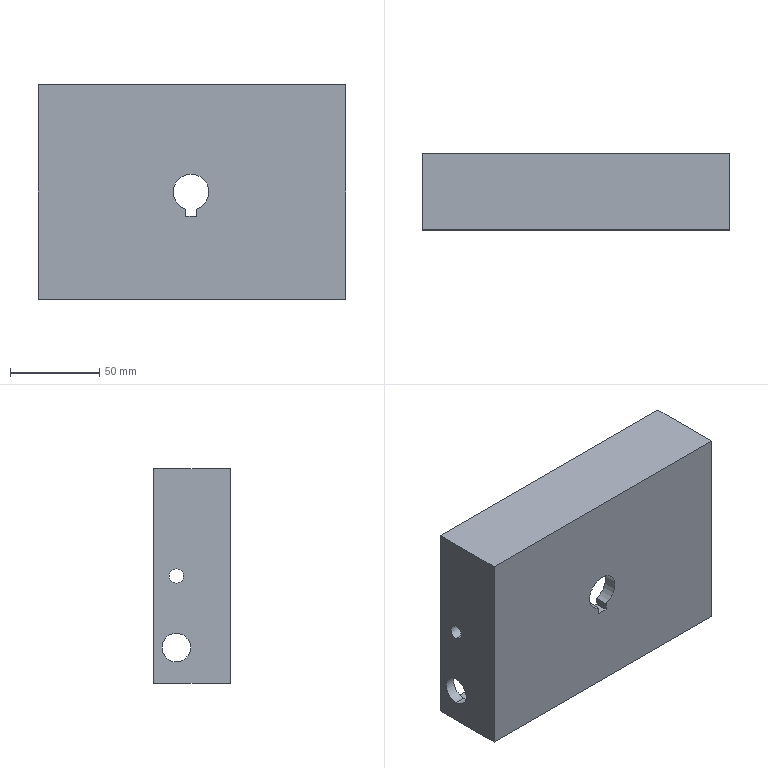Part | SolidWorks | features ICE 3, Extrusion 1 | 1 solid | 23 faces | box 172 x 42.5 x 120 mm | volume 233262 mm3 | plane 14 | cylinder 9 | commonest cylinder face diameters 8 x4 16 x4 20 x1
STEP:
#1=CARTESIAN_POINT('',(86.,8.75,56.));
#2=VERTEX_POINT('',#1);
#3=CARTESIAN_POINT('',(86.,8.75,64.));
#4=VERTEX_POINT('',#3);
#5=CARTESIAN_POINT('',(86.,8.75,60.));
#6=DIRECTION('',(-1.,0.,0.));
#7=DIRECTION('',(0.,0.,1.));
#8=AXIS2_PLACEMENT_3D('',#5,#6,#7);
#9=CIRCLE('',#8,4.);
#10=EDGE_CURVE('',#2,#4,#9,.T.);
#11=ORIENTED_EDGE('',*,*,#10,.F.);
#12=CARTESIAN_POINT('',(80.,8.75,56.));
#13=VERTEX_POINT('',#12);
#14=CARTESIAN_POINT('',(86.,8.75,56.));
#15=DIRECTION('',(-1.,0.,0.));
#16=VECTOR('',#15,1000.);
#17=LINE('',#14,#16);
#18=EDGE_CURVE('',#2,#13,#17,.T.);
#19=ORIENTED_EDGE('',*,*,#18,.T.);
#20=CARTESIAN_POINT('',(80.,8.75,64.));
#21=VERTEX_POINT('',#20);
#22=CARTESIAN_POINT('',(80.,8.75,60.));
#23=DIRECTION('',(1.,0.,0.));
#24=DIRECTION('',(0.,0.,-1.));
#25=AXIS2_PLACEMENT_3D('',#22,#23,#24);
#26=CIRCLE('',#25,4.);
#27=EDGE_CURVE('',#21,#13,#26,.T.);
#28=ORIENTED_EDGE('',*,*,#27,.F.);
#29=CARTESIAN_POINT('',(86.,8.75,64.));
#30=DIRECTION('',(-1.,0.,0.));
#31=VECTOR('',#30,1000.);
#32=LINE('',#29,#31);
#33=EDGE_CURVE('',#4,#21,#32,.T.);
#34=ORIENTED_EDGE('',*,*,#33,.F.);
#35=EDGE_LOOP('',(#11,#19,#28,#34));
#36=FACE_OUTER_BOUND('',#35,.T.);
#37=CARTESIAN_POINT('',(86.,8.75,60.));
#38=DIRECTION('',(-1.,0.,0.));
#39=DIRECTION('',(0.,0.,1.));
#40=AXIS2_PLACEMENT_3D('',#37,#38,#39);
#41=CYLINDRICAL_SURFACE('',#40,4.);
#42=ADVANCED_FACE('',(#36),#41,.F.);
#43=CARTESIAN_POINT('',(86.,8.75,12.));
#44=VERTEX_POINT('',#43);
#45=CARTESIAN_POINT('',(86.,8.75,28.));
#46=VERTEX_POINT('',#45);
#47=CARTESIAN_POINT('',(86.,8.75,20.));
#48=DIRECTION('',(-1.,0.,0.));
#49=DIRECTION('',(0.,0.,1.));
#50=AXIS2_PLACEMENT_3D('',#47,#48,#49);
#51=CIRCLE('',#50,8.);
#52=EDGE_CURVE('',#44,#46,#51,.T.);
#53=ORIENTED_EDGE('',*,*,#52,.F.);
#54=CARTESIAN_POINT('',(80.,8.75,12.));
#55=VERTEX_POINT('',#54);
#56=CARTESIAN_POINT('',(86.,8.75,12.));
#57=DIRECTION('',(-1.,0.,0.));
#58=VECTOR('',#57,1000.);
#59=LINE('',#56,#58);
#60=EDGE_CURVE('',#44,#55,#59,.T.);
#61=ORIENTED_EDGE('',*,*,#60,.T.);
#62=CARTESIAN_POINT('',(80.,8.75,28.));
#63=VERTEX_POINT('',#62);
#64=CARTESIAN_POINT('',(80.,8.75,20.));
#65=DIRECTION('',(1.,0.,0.));
#66=DIRECTION('',(0.,0.,-1.));
#67=AXIS2_PLACEMENT_3D('',#64,#65,#66);
#68=CIRCLE('',#67,8.);
#69=EDGE_CURVE('',#63,#55,#68,.T.);
#70=ORIENTED_EDGE('',*,*,#69,.F.);
#71=CARTESIAN_POINT('',(86.,8.75,28.));
#72=DIRECTION('',(-1.,0.,0.));
#73=VECTOR('',#72,1000.);
#74=LINE('',#71,#73);
#75=EDGE_CURVE('',#46,#63,#74,.T.);
#76=ORIENTED_EDGE('',*,*,#75,.F.);
#77=EDGE_LOOP('',(#53,#61,#70,#76));
#78=FACE_OUTER_BOUND('',#77,.T.);
#79=CARTESIAN_POINT('',(86.,8.75,20.));
#80=DIRECTION('',(-1.,0.,0.));
#81=DIRECTION('',(0.,0.,1.));
#82=AXIS2_PLACEMENT_3D('',#79,#80,#81);
#83=CYLINDRICAL_SURFACE('',#82,8.);
#84=ADVANCED_FACE('',(#78),#83,.F.);
#85=CARTESIAN_POINT('',(-80.,8.75,56.));
#86=VERTEX_POINT('',#85);
#87=CARTESIAN_POINT('',(-80.,8.75,64.));
#88=VERTEX_POINT('',#87);
#89=CARTESIAN_POINT('',(-80.,8.75,60.));
#90=DIRECTION('',(-1.,0.,0.));
#91=DIRECTION('',(0.,0.,1.));
#92=AXIS2_PLACEMENT_3D('',#89,#90,#91);
#93=CIRCLE('',#92,4.);
#94=EDGE_CURVE('',#86,#88,#93,.T.);
#95=ORIENTED_EDGE('',*,*,#94,.F.);
#96=CARTESIAN_POINT('',(-86.,8.75,56.));
#97=VERTEX_POINT('',#96);
#98=CARTESIAN_POINT('',(86.,8.75,56.));
#99=DIRECTION('',(-1.,0.,0.));
#100=VECTOR('',#99,1000.);
#101=LINE('',#98,#100);
#102=EDGE_CURVE('',#86,#97,#101,.T.);
#103=ORIENTED_EDGE('',*,*,#102,.T.);
#104=CARTESIAN_POINT('',(-86.,8.75,64.));
#105=VERTEX_POINT('',#104);
#106=CARTESIAN_POINT('',(-86.,8.75,60.));
#107=DIRECTION('',(-1.,0.,0.));
#108=DIRECTION('',(0.,0.,1.));
#109=AXIS2_PLACEMENT_3D('',#106,#107,#108);
#110=CIRCLE('',#109,4.);
#111=EDGE_CURVE('',#97,#105,#110,.T.);
#112=ORIENTED_EDGE('',*,*,#111,.T.);
#113=CARTESIAN_POINT('',(86.,8.75,64.));
#114=DIRECTION('',(-1.,0.,0.));
#115=VECTOR('',#114,1000.);
#116=LINE('',#113,#115);
#117=EDGE_CURVE('',#88,#105,#116,.T.);
#118=ORIENTED_EDGE('',*,*,#117,.F.);
#119=EDGE_LOOP('',(#95,#103,#112,#118));
#120=FACE_OUTER_BOUND('',#119,.T.);
#121=CARTESIAN_POINT('',(86.,8.75,60.));
#122=DIRECTION('',(-1.,0.,0.));
#123=DIRECTION('',(0.,0.,1.));
#124=AXIS2_PLACEMENT_3D('',#121,#122,#123);
#125=CYLINDRICAL_SURFACE('',#124,4.);
#126=ADVANCED_FACE('',(#120),#125,.F.);
#127=CARTESIAN_POINT('',(-80.,8.75,12.));
#128=VERTEX_POINT('',#127);
#129=CARTESIAN_POINT('',(-80.,8.75,28.));
#130=VERTEX_POINT('',#129);
#131=CARTESIAN_POINT('',(-80.,8.75,20.));
#132=DIRECTION('',(-1.,0.,0.));
#133=DIRECTION('',(0.,0.,1.));
#134=AXIS2_PLACEMENT_3D('',#131,#132,#133);
#135=CIRCLE('',#134,8.);
#136=EDGE_CURVE('',#128,#130,#135,.T.);
#137=ORIENTED_EDGE('',*,*,#136,.F.);
#138=CARTESIAN_POINT('',(-86.,8.75,12.));
#139=VERTEX_POINT('',#138);
#140=CARTESIAN_POINT('',(86.,8.75,12.));
#141=DIRECTION('',(-1.,0.,0.));
#142=VECTOR('',#141,1000.);
#143=LINE('',#140,#142);
#144=EDGE_CURVE('',#128,#139,#143,.T.);
#145=ORIENTED_EDGE('',*,*,#144,.T.);
#146=CARTESIAN_POINT('',(-86.,8.75,28.));
#147=VERTEX_POINT('',#146);
#148=CARTESIAN_POINT('',(-86.,8.75,20.));
#149=DIRECTION('',(-1.,0.,0.));
#150=DIRECTION('',(0.,0.,1.));
#151=AXIS2_PLACEMENT_3D('',#148,#149,#150);
#152=CIRCLE('',#151,8.);
#153=EDGE_CURVE('',#139,#147,#152,.T.);
#154=ORIENTED_EDGE('',*,*,#153,.T.);
#155=CARTESIAN_POINT('',(86.,8.75,28.));
#156=DIRECTION('',(-1.,0.,0.));
#157=VECTOR('',#156,1000.);
#158=LINE('',#155,#157);
#159=EDGE_CURVE('',#130,#147,#158,.T.);
#160=ORIENTED_EDGE('',*,*,#159,.F.);
#161=EDGE_LOOP('',(#137,#145,#154,#160));
#162=FACE_OUTER_BOUND('',#161,.T.);
#163=CARTESIAN_POINT('',(86.,8.75,20.));
#164=DIRECTION('',(-1.,0.,0.));
#165=DIRECTION('',(0.,0.,1.));
#166=AXIS2_PLACEMENT_3D('',#163,#164,#165);
#167=CYLINDRICAL_SURFACE('',#166,8.);
#168=ADVANCED_FACE('',(#162),#167,.F.);
#169=CARTESIAN_POINT('',(86.,8.75,60.));
#170=DIRECTION('',(-1.,0.,0.));
#171=DIRECTION('',(0.,0.,1.));
#172=AXIS2_PLACEMENT_3D('',#169,#170,#171);
#173=CIRCLE('',#172,4.);
#174=EDGE_CURVE('',#4,#2,#173,.T.);
#175=ORIENTED_EDGE('',*,*,#174,.T.);
#176=ORIENTED_EDGE('',*,*,#10,.T.);
#177=EDGE_LOOP('',(#175,#176));
#178=FACE_BOUND('',#177,.T.);
#179=CARTESIAN_POINT('',(86.,8.75,20.));
#180=DIRECTION('',(-1.,0.,0.));
#181=DIRECTION('',(0.,0.,1.));
#182=AXIS2_PLACEMENT_3D('',#179,#180,#181);
#183=CIRCLE('',#182,8.);
#184=EDGE_CURVE('',#46,#44,#183,.T.);
#185=ORIENTED_EDGE('',*,*,#184,.T.);
#186=ORIENTED_EDGE('',*,*,#52,.T.);
#187=EDGE_LOOP('',(#185,#186));
#188=FACE_BOUND('',#187,.T.);
#189=CARTESIAN_POINT('',(86.,-21.25,0.));
#190=VERTEX_POINT('',#189);
#191=CARTESIAN_POINT('',(86.,21.25,0.));
#192=VERTEX_POINT('',#191);
#193=CARTESIAN_POINT('',(86.,-21.25,0.));
#194=DIRECTION('',(0.,1.,0.));
#195=VECTOR('',#194,1000.);
#196=LINE('',#193,#195);
#197=EDGE_CURVE('',#190,#192,#196,.T.);
#198=ORIENTED_EDGE('',*,*,#197,.T.);
#199=CARTESIAN_POINT('',(86.,21.25,120.));
#200=VERTEX_POINT('',#199);
#201=CARTESIAN_POINT('',(86.,21.25,120.));
#202=DIRECTION('',(0.,0.,-1.));
#203=VECTOR('',#202,1000.);
#204=LINE('',#201,#203);
#205=EDGE_CURVE('',#200,#192,#204,.T.);
#206=ORIENTED_EDGE('',*,*,#205,.F.);
#207=CARTESIAN_POINT('',(86.,-21.25,120.));
#208=VERTEX_POINT('',#207);
#209=CARTESIAN_POINT('',(86.,-21.25,120.));
#210=DIRECTION('',(0.,1.,0.));
#211=VECTOR('',#210,1000.);
#212=LINE('',#209,#211);
#213=EDGE_CURVE('',#208,#200,#212,.T.);
#214=ORIENTED_EDGE('',*,*,#213,.F.);
#215=CARTESIAN_POINT('',(86.,-21.25,120.));
#216=DIRECTION('',(0.,0.,-1.));
#217=VECTOR('',#216,1000.);
#218=LINE('',#215,#217);
#219=EDGE_CURVE('',#208,#190,#218,.T.);
#220=ORIENTED_EDGE('',*,*,#219,.T.);
#221=EDGE_LOOP('',(#198,#206,#214,#220));
#222=FACE_OUTER_BOUND('',#221,.T.);
#223=CARTESIAN_POINT('',(86.,-21.25,120.));
#224=DIRECTION('',(-1.,0.,0.));
#225=DIRECTION('',(0.,0.,1.));
#226=AXIS2_PLACEMENT_3D('',#223,#224,#225);
#227=PLANE('',#226);
#228=ADVANCED_FACE('',(#178,#188,#222),#227,.F.);
#229=CARTESIAN_POINT('',(-80.,21.25,3.));
#230=VERTEX_POINT('',#229);
#231=CARTESIAN_POINT('',(-80.,21.25,117.));
#232=VERTEX_POINT('',#231);
#233=CARTESIAN_POINT('',(-80.,21.25,5.));
#234=DIRECTION('',(0.,0.,1.));
#235=VECTOR('',#234,1000.);
#236=LINE('',#233,#235);
#237=EDGE_CURVE('',#230,#232,#236,.T.);
#238=ORIENTED_EDGE('',*,*,#237,.F.);
#239=CARTESIAN_POINT('',(80.,21.25,3.));
#240=VERTEX_POINT('',#239);
#241=CARTESIAN_POINT('',(-80.,21.25,3.));
#242=DIRECTION('',(-1.,0.,0.));
#243=VECTOR('',#242,1000.);
#244=LINE('',#241,#243);
#245=EDGE_CURVE('',#240,#230,#244,.T.);
#246=ORIENTED_EDGE('',*,*,#245,.F.);
#247=CARTESIAN_POINT('',(80.,21.25,117.));
#248=VERTEX_POINT('',#247);
#249=CARTESIAN_POINT('',(80.,21.25,3.));
#250=DIRECTION('',(0.,0.,-1.));
#251=VECTOR('',#250,1000.);
#252=LINE('',#249,#251);
#253=EDGE_CURVE('',#248,#240,#252,.T.);
#254=ORIENTED_EDGE('',*,*,#253,.F.);
#255=CARTESIAN_POINT('',(-80.,21.25,117.));
#256=DIRECTION('',(1.,0.,0.));
#257=VECTOR('',#256,1000.);
#258=LINE('',#255,#257);
#259=EDGE_CURVE('',#232,#248,#258,.T.);
#260=ORIENTED_EDGE('',*,*,#259,.F.);
#261=EDGE_LOOP('',(#238,#246,#254,#260));
#262=FACE_BOUND('',#261,.T.);
#263=CARTESIAN_POINT('',(-86.,21.25,0.));
#264=VERTEX_POINT('',#263);
#265=CARTESIAN_POINT('',(-86.,21.25,0.));
#266=DIRECTION('',(-1.,0.,0.));
#267=VECTOR('',#266,1000.);
#268=LINE('',#265,#267);
#269=EDGE_CURVE('',#192,#264,#268,.T.);
#270=ORIENTED_EDGE('',*,*,#269,.T.);
#271=CARTESIAN_POINT('',(-86.,21.25,120.));
#272=VERTEX_POINT('',#271);
#273=CARTESIAN_POINT('',(-86.,21.25,120.));
#274=DIRECTION('',(0.,0.,-1.));
#275=VECTOR('',#274,1000.);
#276=LINE('',#273,#275);
#277=EDGE_CURVE('',#272,#264,#276,.T.);
#278=ORIENTED_EDGE('',*,*,#277,.F.);
#279=CARTESIAN_POINT('',(-86.,21.25,120.));
#280=DIRECTION('',(-1.,0.,0.));
#281=VECTOR('',#280,1000.);
#282=LINE('',#279,#281);
#283=EDGE_CURVE('',#200,#272,#282,.T.);
#284=ORIENTED_EDGE('',*,*,#283,.F.);
#285=ORIENTED_EDGE('',*,*,#205,.T.);
#286=EDGE_LOOP('',(#270,#278,#284,#285));
#287=FACE_OUTER_BOUND('',#286,.T.);
#288=CARTESIAN_POINT('',(-86.,21.25,120.));
#289=DIRECTION('',(0.,-1.,0.));
#290=DIRECTION('',(0.,0.,-1.));
#291=AXIS2_PLACEMENT_3D('',#288,#289,#290);
#292=PLANE('',#291);
#293=ADVANCED_FACE('',(#262,#287),#292,.F.);
#294=CARTESIAN_POINT('',(-86.,8.75,60.));
#295=DIRECTION('',(-1.,0.,0.));
#296=DIRECTION('',(0.,0.,1.));
#297=AXIS2_PLACEMENT_3D('',#294,#295,#296);
#298=CIRCLE('',#297,4.);
#299=EDGE_CURVE('',#105,#97,#298,.T.);
#300=ORIENTED_EDGE('',*,*,#299,.F.);
#301=ORIENTED_EDGE('',*,*,#111,.F.);
#302=EDGE_LOOP('',(#300,#301));
#303=FACE_BOUND('',#302,.T.);
#304=CARTESIAN_POINT('',(-86.,8.75,20.));
#305=DIRECTION('',(-1.,0.,0.));
#306=DIRECTION('',(0.,0.,1.));
#307=AXIS2_PLACEMENT_3D('',#304,#305,#306);
#308=CIRCLE('',#307,8.);
#309=EDGE_CURVE('',#147,#139,#308,.T.);
#310=ORIENTED_EDGE('',*,*,#309,.F.);
#311=ORIENTED_EDGE('',*,*,#153,.F.);
#312=EDGE_LOOP('',(#310,#311));
#313=FACE_BOUND('',#312,.T.);
#314=CARTESIAN_POINT('',(-86.,-21.25,0.));
#315=VERTEX_POINT('',#314);
#316=CARTESIAN_POINT('',(-86.,-21.25,0.));
#317=DIRECTION('',(0.,-1.,0.));
#318=VECTOR('',#317,1000.);
#319=LINE('',#316,#318);
#320=EDGE_CURVE('',#264,#315,#319,.T.);
#321=ORIENTED_EDGE('',*,*,#320,.T.);
#322=CARTESIAN_POINT('',(-86.,-21.25,120.));
#323=VERTEX_POINT('',#322);
#324=CARTESIAN_POINT('',(-86.,-21.25,120.));
#325=DIRECTION('',(0.,0.,-1.));
#326=VECTOR('',#325,1000.);
#327=LINE('',#324,#326);
#328=EDGE_CURVE('',#323,#315,#327,.T.);
#329=ORIENTED_EDGE('',*,*,#328,.F.);
#330=CARTESIAN_POINT('',(-86.,-21.25,120.));
#331=DIRECTION('',(0.,-1.,0.));
#332=VECTOR('',#331,1000.);
#333=LINE('',#330,#332);
#334=EDGE_CURVE('',#272,#323,#333,.T.);
#335=ORIENTED_EDGE('',*,*,#334,.F.);
#336=ORIENTED_EDGE('',*,*,#277,.T.);
#337=EDGE_LOOP('',(#321,#329,#335,#336));
#338=FACE_OUTER_BOUND('',#337,.T.);
#339=CARTESIAN_POINT('',(-86.,-21.25,120.));
#340=DIRECTION('',(1.,0.,0.));
#341=DIRECTION('',(0.,0.,-1.));
#342=AXIS2_PLACEMENT_3D('',#339,#340,#341);
#343=PLANE('',#342);
#344=ADVANCED_FACE('',(#303,#313,#338),#343,.F.);
#345=CARTESIAN_POINT('',(-3.518,-21.25,50.461));
#346=VERTEX_POINT('',#345);
#347=CARTESIAN_POINT('',(-3.518,-21.25,46.461));
#348=VERTEX_POINT('',#347);
#349=CARTESIAN_POINT('',(-3.518,-21.25,50.461));
#350=DIRECTION('',(0.,0.,-1.));
#351=VECTOR('',#350,1000.);
#352=LINE('',#349,#351);
#353=EDGE_CURVE('',#346,#348,#352,.T.);
#354=ORIENTED_EDGE('',*,*,#353,.F.);
#355=CARTESIAN_POINT('',(2.482,-21.25,50.461));
#356=VERTEX_POINT('',#355);
#357=CARTESIAN_POINT('',(-0.5176,-21.25,60.));
#358=DIRECTION('',(0.,-1.,0.));
#359=DIRECTION('',(0.,0.,-1.));
#360=AXIS2_PLACEMENT_3D('',#357,#358,#359);
#361=CIRCLE('',#360,10.);
#362=EDGE_CURVE('',#356,#346,#361,.T.);
#363=ORIENTED_EDGE('',*,*,#362,.F.);
#364=CARTESIAN_POINT('',(2.482,-21.25,46.461));
#365=VERTEX_POINT('',#364);
#366=CARTESIAN_POINT('',(2.482,-21.25,46.461));
#367=DIRECTION('',(0.,0.,1.));
#368=VECTOR('',#367,1000.);
#369=LINE('',#366,#368);
#370=EDGE_CURVE('',#365,#356,#369,.T.);
#371=ORIENTED_EDGE('',*,*,#370,.F.);
#372=CARTESIAN_POINT('',(-3.518,-21.25,46.461));
#373=DIRECTION('',(1.,0.,0.));
#374=VECTOR('',#373,1000.);
#375=LINE('',#372,#374);
#376=EDGE_CURVE('',#348,#365,#375,.T.);
#377=ORIENTED_EDGE('',*,*,#376,.F.);
#378=EDGE_LOOP('',(#354,#363,#371,#377));
#379=FACE_BOUND('',#378,.T.);
#380=CARTESIAN_POINT('',(-86.,-21.25,0.));
#381=DIRECTION('',(1.,0.,0.));
#382=VECTOR('',#381,1000.);
#383=LINE('',#380,#382);
#384=EDGE_CURVE('',#315,#190,#383,.T.);
#385=ORIENTED_EDGE('',*,*,#384,.T.);
#386=ORIENTED_EDGE('',*,*,#219,.F.);
#387=CARTESIAN_POINT('',(-86.,-21.25,120.));
#388=DIRECTION('',(1.,0.,0.));
#389=VECTOR('',#388,1000.);
#390=LINE('',#387,#389);
#391=EDGE_CURVE('',#323,#208,#390,.T.);
#392=ORIENTED_EDGE('',*,*,#391,.F.);
#393=ORIENTED_EDGE('',*,*,#328,.T.);
#394=EDGE_LOOP('',(#385,#386,#392,#393));
#395=FACE_OUTER_BOUND('',#394,.T.);
#396=CARTESIAN_POINT('',(-86.,-21.25,120.));
#397=DIRECTION('',(0.,1.,0.));
#398=DIRECTION('',(0.,0.,1.));
#399=AXIS2_PLACEMENT_3D('',#396,#397,#398);
#400=PLANE('',#399);
#401=ADVANCED_FACE('',(#379,#395),#400,.F.);
#402=ORIENTED_EDGE('',*,*,#213,.T.);
#403=ORIENTED_EDGE('',*,*,#283,.T.);
#404=ORIENTED_EDGE('',*,*,#334,.T.);
#405=ORIENTED_EDGE('',*,*,#391,.T.);
#406=EDGE_LOOP('',(#402,#403,#404,#405));
#407=FACE_OUTER_BOUND('',#406,.T.);
#408=CARTESIAN_POINT('',(0.,0.,120.));
#409=DIRECTION('',(0.,0.,-1.));
#410=DIRECTION('',(-1.,0.,0.));
#411=AXIS2_PLACEMENT_3D('',#408,#409,#410);
#412=PLANE('',#411);
#413=ADVANCED_FACE('',(#407),#412,.F.);
#414=ORIENTED_EDGE('',*,*,#197,.F.);
#415=ORIENTED_EDGE('',*,*,#384,.F.);
#416=ORIENTED_EDGE('',*,*,#320,.F.);
#417=ORIENTED_EDGE('',*,*,#269,.F.);
#418=EDGE_LOOP('',(#414,#415,#416,#417));
#419=FACE_OUTER_BOUND('',#418,.T.);
#420=CARTESIAN_POINT('',(0.,0.,0.));
#421=DIRECTION('',(0.,0.,-1.));
#422=DIRECTION('',(-1.,0.,0.));
#423=AXIS2_PLACEMENT_3D('',#420,#421,#422);
#424=PLANE('',#423);
#425=ADVANCED_FACE('',(#419),#424,.T.);
#426=ORIENTED_EDGE('',*,*,#245,.T.);
#427=CARTESIAN_POINT('',(-80.,-13.75,3.));
#428=VERTEX_POINT('',#427);
#429=CARTESIAN_POINT('',(-80.,-13.75,3.));
#430=DIRECTION('',(0.,1.,0.));
#431=VECTOR('',#430,1000.);
#432=LINE('',#429,#431);
#433=EDGE_CURVE('',#428,#230,#432,.T.);
#434=ORIENTED_EDGE('',*,*,#433,.F.);
#435=CARTESIAN_POINT('',(80.,-13.75,3.));
#436=VERTEX_POINT('',#435);
#437=CARTESIAN_POINT('',(-80.,-13.75,3.));
#438=DIRECTION('',(-1.,0.,0.));
#439=VECTOR('',#438,1000.);
#440=LINE('',#437,#439);
#441=EDGE_CURVE('',#436,#428,#440,.T.);
#442=ORIENTED_EDGE('',*,*,#441,.F.);
#443=CARTESIAN_POINT('',(80.,-13.75,3.));
#444=DIRECTION('',(0.,1.,0.));
#445=VECTOR('',#444,1000.);
#446=LINE('',#443,#445);
#447=EDGE_CURVE('',#436,#240,#446,.T.);
#448=ORIENTED_EDGE('',*,*,#447,.T.);
#449=EDGE_LOOP('',(#426,#434,#442,#448));
#450=FACE_OUTER_BOUND('',#449,.T.);
#451=CARTESIAN_POINT('',(-80.,-13.75,3.));
#452=DIRECTION('',(0.,0.,-1.));
#453=DIRECTION('',(-1.,0.,0.));
#454=AXIS2_PLACEMENT_3D('',#451,#452,#453);
#455=PLANE('',#454);
#456=ADVANCED_FACE('',(#450),#455,.F.);
#457=ORIENTED_EDGE('',*,*,#27,.T.);
#458=CARTESIAN_POINT('',(80.,8.75,60.));
#459=DIRECTION('',(1.,0.,0.));
#460=DIRECTION('',(0.,0.,-1.));
#461=AXIS2_PLACEMENT_3D('',#458,#459,#460);
#462=CIRCLE('',#461,4.);
#463=EDGE_CURVE('',#13,#21,#462,.T.);
#464=ORIENTED_EDGE('',*,*,#463,.T.);
#465=EDGE_LOOP('',(#457,#464));
#466=FACE_BOUND('',#465,.T.);
#467=ORIENTED_EDGE('',*,*,#69,.T.);
#468=CARTESIAN_POINT('',(80.,8.75,20.));
#469=DIRECTION('',(1.,0.,0.));
#470=DIRECTION('',(0.,0.,-1.));
#471=AXIS2_PLACEMENT_3D('',#468,#469,#470);
#472=CIRCLE('',#471,8.);
#473=EDGE_CURVE('',#55,#63,#472,.T.);
#474=ORIENTED_EDGE('',*,*,#473,.T.);
#475=EDGE_LOOP('',(#467,#474));
#476=FACE_BOUND('',#475,.T.);
#477=ORIENTED_EDGE('',*,*,#253,.T.);
#478=ORIENTED_EDGE('',*,*,#447,.F.);
#479=CARTESIAN_POINT('',(80.,-13.75,117.));
#480=VERTEX_POINT('',#479);
#481=CARTESIAN_POINT('',(80.,-13.75,5.));
#482=DIRECTION('',(0.,0.,-1.));
#483=VECTOR('',#482,1000.);
#484=LINE('',#481,#483);
#485=EDGE_CURVE('',#480,#436,#484,.T.);
#486=ORIENTED_EDGE('',*,*,#485,.F.);
#487=CARTESIAN_POINT('',(80.,-13.75,117.));
#488=DIRECTION('',(0.,1.,0.));
#489=VECTOR('',#488,1000.);
#490=LINE('',#487,#489);
#491=EDGE_CURVE('',#480,#248,#490,.T.);
#492=ORIENTED_EDGE('',*,*,#491,.T.);
#493=EDGE_LOOP('',(#477,#478,#486,#492));
#494=FACE_OUTER_BOUND('',#493,.T.);
#495=CARTESIAN_POINT('',(80.,-13.75,3.));
#496=DIRECTION('',(1.,0.,0.));
#497=DIRECTION('',(0.,0.,-1.));
#498=AXIS2_PLACEMENT_3D('',#495,#496,#497);
#499=PLANE('',#498);
#500=ADVANCED_FACE('',(#466,#476,#494),#499,.F.);
#501=ORIENTED_EDGE('',*,*,#259,.T.);
#502=ORIENTED_EDGE('',*,*,#491,.F.);
#503=CARTESIAN_POINT('',(-80.,-13.75,117.));
#504=VERTEX_POINT('',#503);
#505=CARTESIAN_POINT('',(-80.,-13.75,117.));
#506=DIRECTION('',(1.,0.,0.));
#507=VECTOR('',#506,1000.);
#508=LINE('',#505,#507);
#509=EDGE_CURVE('',#504,#480,#508,.T.);
#510=ORIENTED_EDGE('',*,*,#509,.F.);
#511=CARTESIAN_POINT('',(-80.,-13.75,117.));
#512=DIRECTION('',(0.,1.,0.));
#513=VECTOR('',#512,1000.);
#514=LINE('',#511,#513);
#515=EDGE_CURVE('',#504,#232,#514,.T.);
#516=ORIENTED_EDGE('',*,*,#515,.T.);
#517=EDGE_LOOP('',(#501,#502,#510,#516));
#518=FACE_OUTER_BOUND('',#517,.T.);
#519=CARTESIAN_POINT('',(-80.,-13.75,117.));
#520=DIRECTION('',(0.,0.,1.));
#521=DIRECTION('',(1.,0.,0.));
#522=AXIS2_PLACEMENT_3D('',#519,#520,#521);
#523=PLANE('',#522);
#524=ADVANCED_FACE('',(#518),#523,.F.);
#525=CARTESIAN_POINT('',(-80.,8.75,60.));
#526=DIRECTION('',(-1.,0.,0.));
#527=DIRECTION('',(0.,0.,1.));
#528=AXIS2_PLACEMENT_3D('',#525,#526,#527);
#529=CIRCLE('',#528,4.);
#530=EDGE_CURVE('',#88,#86,#529,.T.);
#531=ORIENTED_EDGE('',*,*,#530,.T.);
#532=ORIENTED_EDGE('',*,*,#94,.T.);
#533=EDGE_LOOP('',(#531,#532));
#534=FACE_BOUND('',#533,.T.);
#535=CARTESIAN_POINT('',(-80.,8.75,20.));
#536=DIRECTION('',(-1.,0.,0.));
#537=DIRECTION('',(0.,0.,1.));
#538=AXIS2_PLACEMENT_3D('',#535,#536,#537);
#539=CIRCLE('',#538,8.);
#540=EDGE_CURVE('',#130,#128,#539,.T.);
#541=ORIENTED_EDGE('',*,*,#540,.T.);
#542=ORIENTED_EDGE('',*,*,#136,.T.);
#543=EDGE_LOOP('',(#541,#542));
#544=FACE_BOUND('',#543,.T.);
#545=ORIENTED_EDGE('',*,*,#237,.T.);
#546=ORIENTED_EDGE('',*,*,#515,.F.);
#547=CARTESIAN_POINT('',(-80.,-13.75,5.));
#548=DIRECTION('',(0.,0.,1.));
#549=VECTOR('',#548,1000.);
#550=LINE('',#547,#549);
#551=EDGE_CURVE('',#428,#504,#550,.T.);
#552=ORIENTED_EDGE('',*,*,#551,.F.);
#553=ORIENTED_EDGE('',*,*,#433,.T.);
#554=EDGE_LOOP('',(#545,#546,#552,#553));
#555=FACE_OUTER_BOUND('',#554,.T.);
#556=CARTESIAN_POINT('',(-80.,-13.75,5.));
#557=DIRECTION('',(-1.,0.,0.));
#558=DIRECTION('',(0.,0.,1.));
#559=AXIS2_PLACEMENT_3D('',#556,#557,#558);
#560=PLANE('',#559);
#561=ADVANCED_FACE('',(#534,#544,#555),#560,.F.);
#562=CARTESIAN_POINT('',(2.482,-13.75,46.461));
#563=VERTEX_POINT('',#562);
#564=CARTESIAN_POINT('',(2.482,-13.75,50.461));
#565=VERTEX_POINT('',#564);
#566=CARTESIAN_POINT('',(2.482,-13.75,0.));
#567=DIRECTION('',(0.,0.,1.));
#568=VECTOR('',#567,1000.);
#569=LINE('',#566,#568);
#570=EDGE_CURVE('',#563,#565,#569,.T.);
#571=ORIENTED_EDGE('',*,*,#570,.T.);
#572=CARTESIAN_POINT('',(-3.518,-13.75,50.461));
#573=VERTEX_POINT('',#572);
#574=CARTESIAN_POINT('',(-0.5176,-13.75,60.));
#575=DIRECTION('',(0.,-1.,0.));
#576=DIRECTION('',(0.,0.,-1.));
#577=AXIS2_PLACEMENT_3D('',#574,#575,#576);
#578=CIRCLE('',#577,10.);
#579=EDGE_CURVE('',#565,#573,#578,.T.);
#580=ORIENTED_EDGE('',*,*,#579,.T.);
#581=CARTESIAN_POINT('',(-3.518,-13.75,46.461));
#582=VERTEX_POINT('',#581);
#583=CARTESIAN_POINT('',(-3.518,-13.75,0.));
#584=DIRECTION('',(0.,0.,-1.));
#585=VECTOR('',#584,1000.);
#586=LINE('',#583,#585);
#587=EDGE_CURVE('',#573,#582,#586,.T.);
#588=ORIENTED_EDGE('',*,*,#587,.T.);
#589=CARTESIAN_POINT('',(0.,-13.75,46.461));
#590=DIRECTION('',(1.,0.,0.));
#591=VECTOR('',#590,1000.);
#592=LINE('',#589,#591);
#593=EDGE_CURVE('',#582,#563,#592,.T.);
#594=ORIENTED_EDGE('',*,*,#593,.T.);
#595=EDGE_LOOP('',(#571,#580,#588,#594));
#596=FACE_BOUND('',#595,.T.);
#597=ORIENTED_EDGE('',*,*,#441,.T.);
#598=ORIENTED_EDGE('',*,*,#551,.T.);
#599=ORIENTED_EDGE('',*,*,#509,.T.);
#600=ORIENTED_EDGE('',*,*,#485,.T.);
#601=EDGE_LOOP('',(#597,#598,#599,#600));
#602=FACE_OUTER_BOUND('',#601,.T.);
#603=CARTESIAN_POINT('',(0.,-13.75,0.));
#604=DIRECTION('',(0.,-1.,0.));
#605=DIRECTION('',(0.,0.,-1.));
#606=AXIS2_PLACEMENT_3D('',#603,#604,#605);
#607=PLANE('',#606);
#608=ADVANCED_FACE('',(#596,#602),#607,.F.);
#609=ORIENTED_EDGE('',*,*,#144,.F.);
#610=ORIENTED_EDGE('',*,*,#540,.F.);
#611=ORIENTED_EDGE('',*,*,#159,.T.);
#612=ORIENTED_EDGE('',*,*,#309,.T.);
#613=EDGE_LOOP('',(#609,#610,#611,#612));
#614=FACE_OUTER_BOUND('',#613,.T.);
#615=CARTESIAN_POINT('',(86.,8.75,20.));
#616=DIRECTION('',(-1.,0.,0.));
#617=DIRECTION('',(0.,0.,1.));
#618=AXIS2_PLACEMENT_3D('',#615,#616,#617);
#619=CYLINDRICAL_SURFACE('',#618,8.);
#620=ADVANCED_FACE('',(#614),#619,.F.);
#621=ORIENTED_EDGE('',*,*,#102,.F.);
#622=ORIENTED_EDGE('',*,*,#530,.F.);
#623=ORIENTED_EDGE('',*,*,#117,.T.);
#624=ORIENTED_EDGE('',*,*,#299,.T.);
#625=EDGE_LOOP('',(#621,#622,#623,#624));
#626=FACE_OUTER_BOUND('',#625,.T.);
#627=CARTESIAN_POINT('',(86.,8.75,60.));
#628=DIRECTION('',(-1.,0.,0.));
#629=DIRECTION('',(0.,0.,1.));
#630=AXIS2_PLACEMENT_3D('',#627,#628,#629);
#631=CYLINDRICAL_SURFACE('',#630,4.);
#632=ADVANCED_FACE('',(#626),#631,.F.);
#633=ORIENTED_EDGE('',*,*,#60,.F.);
#634=ORIENTED_EDGE('',*,*,#184,.F.);
#635=ORIENTED_EDGE('',*,*,#75,.T.);
#636=ORIENTED_EDGE('',*,*,#473,.F.);
#637=EDGE_LOOP('',(#633,#634,#635,#636));
#638=FACE_OUTER_BOUND('',#637,.T.);
#639=CARTESIAN_POINT('',(86.,8.75,20.));
#640=DIRECTION('',(-1.,0.,0.));
#641=DIRECTION('',(0.,0.,1.));
#642=AXIS2_PLACEMENT_3D('',#639,#640,#641);
#643=CYLINDRICAL_SURFACE('',#642,8.);
#644=ADVANCED_FACE('',(#638),#643,.F.);
#645=ORIENTED_EDGE('',*,*,#18,.F.);
#646=ORIENTED_EDGE('',*,*,#174,.F.);
#647=ORIENTED_EDGE('',*,*,#33,.T.);
#648=ORIENTED_EDGE('',*,*,#463,.F.);
#649=EDGE_LOOP('',(#645,#646,#647,#648));
#650=FACE_OUTER_BOUND('',#649,.T.);
#651=CARTESIAN_POINT('',(86.,8.75,60.));
#652=DIRECTION('',(-1.,0.,0.));
#653=DIRECTION('',(0.,0.,1.));
#654=AXIS2_PLACEMENT_3D('',#651,#652,#653);
#655=CYLINDRICAL_SURFACE('',#654,4.);
#656=ADVANCED_FACE('',(#650),#655,.F.);
#657=CARTESIAN_POINT('',(2.482,21.25,50.461));
#658=DIRECTION('',(0.,-1.,0.));
#659=VECTOR('',#658,1000.);
#660=LINE('',#657,#659);
#661=EDGE_CURVE('',#565,#356,#660,.T.);
#662=ORIENTED_EDGE('',*,*,#661,.T.);
#663=ORIENTED_EDGE('',*,*,#362,.T.);
#664=CARTESIAN_POINT('',(-3.518,21.25,50.461));
#665=DIRECTION('',(0.,-1.,0.));
#666=VECTOR('',#665,1000.);
#667=LINE('',#664,#666);
#668=EDGE_CURVE('',#573,#346,#667,.T.);
#669=ORIENTED_EDGE('',*,*,#668,.F.);
#670=ORIENTED_EDGE('',*,*,#579,.F.);
#671=EDGE_LOOP('',(#662,#663,#669,#670));
#672=FACE_OUTER_BOUND('',#671,.T.);
#673=CARTESIAN_POINT('',(-0.5176,21.25,60.));
#674=DIRECTION('',(0.,-1.,0.));
#675=DIRECTION('',(0.,0.,-1.));
#676=AXIS2_PLACEMENT_3D('',#673,#674,#675);
#677=CYLINDRICAL_SURFACE('',#676,10.);
#678=ADVANCED_FACE('',(#672),#677,.F.);
#679=CARTESIAN_POINT('',(2.482,21.25,46.461));
#680=DIRECTION('',(0.,-1.,0.));
#681=VECTOR('',#680,1000.);
#682=LINE('',#679,#681);
#683=EDGE_CURVE('',#563,#365,#682,.T.);
#684=ORIENTED_EDGE('',*,*,#683,.T.);
#685=ORIENTED_EDGE('',*,*,#370,.T.);
#686=ORIENTED_EDGE('',*,*,#661,.F.);
#687=ORIENTED_EDGE('',*,*,#570,.F.);
#688=EDGE_LOOP('',(#684,#685,#686,#687));
#689=FACE_OUTER_BOUND('',#688,.T.);
#690=CARTESIAN_POINT('',(2.482,21.25,46.461));
#691=DIRECTION('',(1.,0.,0.));
#692=DIRECTION('',(0.,0.,-1.));
#693=AXIS2_PLACEMENT_3D('',#690,#691,#692);
#694=PLANE('',#693);
#695=ADVANCED_FACE('',(#689),#694,.F.);
#696=CARTESIAN_POINT('',(-3.518,21.25,46.461));
#697=DIRECTION('',(0.,-1.,0.));
#698=VECTOR('',#697,1000.);
#699=LINE('',#696,#698);
#700=EDGE_CURVE('',#582,#348,#699,.T.);
#701=ORIENTED_EDGE('',*,*,#700,.T.);
#702=ORIENTED_EDGE('',*,*,#376,.T.);
#703=ORIENTED_EDGE('',*,*,#683,.F.);
#704=ORIENTED_EDGE('',*,*,#593,.F.);
#705=EDGE_LOOP('',(#701,#702,#703,#704));
#706=FACE_OUTER_BOUND('',#705,.T.);
#707=CARTESIAN_POINT('',(-3.518,21.25,46.461));
#708=DIRECTION('',(0.,0.,-1.));
#709=DIRECTION('',(-1.,0.,0.));
#710=AXIS2_PLACEMENT_3D('',#707,#708,#709);
#711=PLANE('',#710);
#712=ADVANCED_FACE('',(#706),#711,.F.);
#713=ORIENTED_EDGE('',*,*,#668,.T.);
#714=ORIENTED_EDGE('',*,*,#353,.T.);
#715=ORIENTED_EDGE('',*,*,#700,.F.);
#716=ORIENTED_EDGE('',*,*,#587,.F.);
#717=EDGE_LOOP('',(#713,#714,#715,#716));
#718=FACE_OUTER_BOUND('',#717,.T.);
#719=CARTESIAN_POINT('',(-3.518,21.25,50.461));
#720=DIRECTION('',(-1.,0.,0.));
#721=DIRECTION('',(0.,0.,1.));
#722=AXIS2_PLACEMENT_3D('',#719,#720,#721);
#723=PLANE('',#722);
#724=ADVANCED_FACE('',(#718),#723,.F.);
#725=CLOSED_SHELL('',(#42,#84,#126,#168,#228,#293,#344,#401,#413,#425,#456,#500,#524,#561,#608,#620,#632,#644,#656,#678,#695,#712,#724));
#726=MANIFOLD_SOLID_BREP('',#725);
#727=CARTESIAN_POINT('',(0.,0.,0.));
#728=DIRECTION('',(0.,0.,1.));
#729=DIRECTION('',(1.,0.,0.));
#730=AXIS2_PLACEMENT_3D('',#727,#728,#729);
#731=(LENGTH_UNIT()NAMED_UNIT(*)SI_UNIT(.MILLI.,.METRE.));
#732=UNCERTAINTY_MEASURE_WITH_UNIT(LENGTH_MEASURE(0.00001),#731,'','');
#733=(NAMED_UNIT(*)PLANE_ANGLE_UNIT()SI_UNIT($,.RADIAN.));
#734=(NAMED_UNIT(*)SI_UNIT($,.STERADIAN.)SOLID_ANGLE_UNIT());
#735=(GEOMETRIC_REPRESENTATION_CONTEXT(3)GLOBAL_UNCERTAINTY_ASSIGNED_CONTEXT((#732))GLOBAL_UNIT_ASSIGNED_CONTEXT((#731,#733,#734))REPRESENTATION_CONTEXT('',''));
#736=ADVANCED_BREP_SHAPE_REPRESENTATION('',(#726,#730),#735);